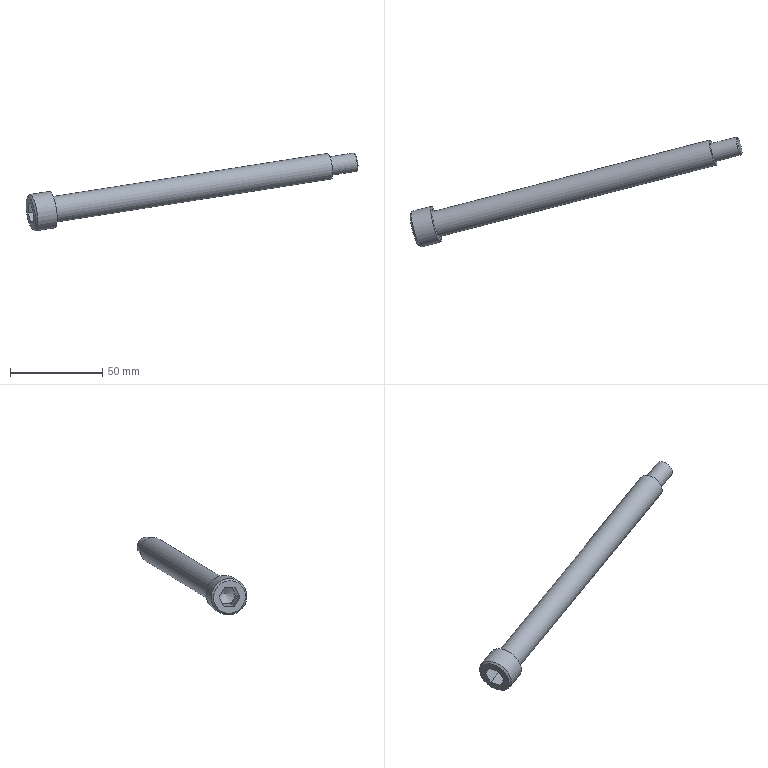Part | STEP file | 车灯-后视镜_id250_x_t | 1 solid | 23 faces | box 180.044 x 59.602 x 42.214 mm | volume 28311 mm3 | plane 17 | cylinder 3 | cone 3 | commonest cylinder face diameters 10 x1 14 x1 20 x1
STEP:
#1=CARTESIAN_POINT('',(-70.664,50.819,2.468));
#2=VERTEX_POINT('',#1);
#3=CARTESIAN_POINT('',(-69.54,46.461,2.468));
#4=DIRECTION('',(0.9573,0.2469,0.1502));
#5=DIRECTION('',(-0.2498,0.9683,0.));
#6=AXIS2_PLACEMENT_3D('',#3,#4,#5);
#7=CIRCLE('',#6,4.5);
#8=EDGE_CURVE('',#2,#2,#7,.T.);
#9=ORIENTED_EDGE('',*,*,#8,.T.);
#10=EDGE_LOOP('',(#9));
#11=FACE_OUTER_BOUND('',#10,.T.);
#12=CARTESIAN_POINT('',(-69.54,46.461,2.468));
#13=DIRECTION('',(0.9573,0.2469,0.1502));
#14=DIRECTION('',(-0.2498,0.9683,0.));
#15=AXIS2_PLACEMENT_3D('',#12,#13,#14);
#16=PLANE('',#15);
#17=ADVANCED_FACE('',(#11),#16,.T.);
#18=CARTESIAN_POINT('',(-85.149,47.599,0.216));
#19=VERTEX_POINT('',#18);
#20=CARTESIAN_POINT('',(-83.9,42.757,0.216));
#21=DIRECTION('',(-0.9573,-0.2469,-0.1502));
#22=DIRECTION('',(-0.2498,0.9683,0.));
#23=AXIS2_PLACEMENT_3D('',#20,#21,#22);
#24=CIRCLE('',#23,5.);
#25=EDGE_CURVE('',#19,#19,#24,.T.);
#26=ORIENTED_EDGE('',*,*,#25,.F.);
#27=EDGE_LOOP('',(#26));
#28=FACE_BOUND('',#27,.T.);
#29=CARTESIAN_POINT('',(-71.267,51.179,2.393));
#30=VERTEX_POINT('',#29);
#31=CARTESIAN_POINT('',(-70.019,46.338,2.393));
#32=DIRECTION('',(-0.9573,-0.2469,-0.1502));
#33=DIRECTION('',(-0.2498,0.9683,0.));
#34=AXIS2_PLACEMENT_3D('',#31,#32,#33);
#35=CIRCLE('',#34,5.);
#36=EDGE_CURVE('',#30,#30,#35,.T.);
#37=ORIENTED_EDGE('',*,*,#36,.T.);
#38=EDGE_LOOP('',(#37));
#39=FACE_BOUND('',#38,.T.);
#40=CARTESIAN_POINT('',(-88.686,41.523,-0.5348));
#41=DIRECTION('',(0.9573,0.2469,0.1502));
#42=DIRECTION('',(-0.2498,0.9683,0.));
#43=AXIS2_PLACEMENT_3D('',#40,#41,#42);
#44=CYLINDRICAL_SURFACE('',#43,5.);
#45=ADVANCED_FACE('',(#28,#39),#44,.T.);
#46=ORIENTED_EDGE('',*,*,#8,.F.);
#47=EDGE_LOOP('',(#46));
#48=FACE_BOUND('',#47,.T.);
#49=ORIENTED_EDGE('',*,*,#36,.F.);
#50=EDGE_LOOP('',(#49));
#51=FACE_BOUND('',#50,.T.);
#52=CARTESIAN_POINT('',(-70.019,46.338,2.393));
#53=DIRECTION('',(-0.9573,-0.2469,-0.1502));
#54=DIRECTION('',(0.2498,-0.9683,0.));
#55=AXIS2_PLACEMENT_3D('',#52,#53,#54);
#56=CONICAL_SURFACE('',#55,5.,45.);
#57=ADVANCED_FACE('',(#48,#51),#56,.T.);
#58=ORIENTED_EDGE('',*,*,#25,.T.);
#59=EDGE_LOOP('',(#58));
#60=FACE_BOUND('',#59,.T.);
#61=CARTESIAN_POINT('',(-85.648,49.535,0.216));
#62=VERTEX_POINT('',#61);
#63=CARTESIAN_POINT('',(-83.9,42.757,0.216));
#64=DIRECTION('',(-0.9573,-0.2469,-0.1502));
#65=DIRECTION('',(-0.2498,0.9683,0.));
#66=AXIS2_PLACEMENT_3D('',#63,#64,#65);
#67=CIRCLE('',#66,7.);
#68=EDGE_CURVE('',#62,#62,#67,.T.);
#69=ORIENTED_EDGE('',*,*,#68,.F.);
#70=EDGE_LOOP('',(#69));
#71=FACE_BOUND('',#70,.T.);
#72=CARTESIAN_POINT('',(-83.9,42.757,0.216));
#73=DIRECTION('',(0.9573,0.2469,0.1502));
#74=DIRECTION('',(-0.2498,0.9683,0.));
#75=AXIS2_PLACEMENT_3D('',#72,#73,#74);
#76=PLANE('',#75);
#77=ADVANCED_FACE('',(#60,#71),#76,.T.);
#78=CARTESIAN_POINT('',(-235.949,10.767,-23.358));
#79=VERTEX_POINT('',#78);
#80=CARTESIAN_POINT('',(-232.452,-2.79,-23.36));
#81=VERTEX_POINT('',#80);
#82=CARTESIAN_POINT('',(-234.2,3.988,-23.359));
#83=DIRECTION('',(0.9573,0.2469,0.1502));
#84=DIRECTION('',(-0.2498,0.9683,0.));
#85=AXIS2_PLACEMENT_3D('',#82,#83,#84);
#86=CIRCLE('',#85,7.);
#87=EDGE_CURVE('',#79,#81,#86,.T.);
#88=ORIENTED_EDGE('',*,*,#87,.T.);
#89=CARTESIAN_POINT('',(-234.2,3.988,-23.359));
#90=DIRECTION('',(0.9576,0.247,0.1481));
#91=DIRECTION('',(0.1433,0.03713,-0.989));
#92=AXIS2_PLACEMENT_3D('',#89,#90,#91);
#93=ELLIPSE('',#92,7.,7.);
#94=EDGE_CURVE('',#81,#79,#93,.T.);
#95=ORIENTED_EDGE('',*,*,#94,.T.);
#96=EDGE_LOOP('',(#88,#95));
#97=FACE_BOUND('',#96,.T.);
#98=ORIENTED_EDGE('',*,*,#68,.T.);
#99=EDGE_LOOP('',(#98));
#100=FACE_BOUND('',#99,.T.);
#101=CARTESIAN_POINT('',(-88.686,41.523,-0.5348));
#102=DIRECTION('',(-0.9573,-0.2469,-0.1502));
#103=DIRECTION('',(0.2498,-0.9683,0.));
#104=AXIS2_PLACEMENT_3D('',#101,#102,#103);
#105=CYLINDRICAL_SURFACE('',#104,7.);
#106=ADVANCED_FACE('',(#97,#100),#105,.T.);
#107=CARTESIAN_POINT('',(-236.698,13.671,-23.358));
#108=VERTEX_POINT('',#107);
#109=CARTESIAN_POINT('',(-231.702,-5.695,-23.361));
#110=VERTEX_POINT('',#109);
#111=CARTESIAN_POINT('',(-234.2,3.988,-23.359));
#112=DIRECTION('',(-0.9576,-0.247,-0.1481));
#113=DIRECTION('',(-0.2498,0.9683,-0.00001827));
#114=AXIS2_PLACEMENT_3D('',#111,#112,#113);
#115=CIRCLE('',#114,10.);
#116=EDGE_CURVE('',#108,#110,#115,.T.);
#117=ORIENTED_EDGE('',*,*,#116,.F.);
#118=CARTESIAN_POINT('',(-234.2,3.988,-23.359));
#119=DIRECTION('',(0.2498,-0.9683,-0.0001518));
#120=VECTOR('',#119,1.);
#121=LINE('',#118,#120);
#122=EDGE_CURVE('',#108,#79,#121,.T.);
#123=ORIENTED_EDGE('',*,*,#122,.T.);
#124=ORIENTED_EDGE('',*,*,#94,.F.);
#125=CARTESIAN_POINT('',(-234.2,3.988,-23.359));
#126=DIRECTION('',(0.2498,-0.9683,-0.0001518));
#127=VECTOR('',#126,1.);
#128=LINE('',#125,#127);
#129=EDGE_CURVE('',#81,#110,#128,.T.);
#130=ORIENTED_EDGE('',*,*,#129,.T.);
#131=EDGE_LOOP('',(#117,#123,#124,#130));
#132=FACE_OUTER_BOUND('',#131,.T.);
#133=CARTESIAN_POINT('',(-234.2,3.988,-23.359));
#134=DIRECTION('',(0.9576,0.247,0.1481));
#135=DIRECTION('',(-0.2498,0.9683,-0.00001827));
#136=AXIS2_PLACEMENT_3D('',#133,#134,#135);
#137=PLANE('',#136);
#138=ADVANCED_FACE('',(#132),#137,.T.);
#139=CARTESIAN_POINT('',(-242.236,-8.412,-24.988));
#140=VERTEX_POINT('',#139);
#141=CARTESIAN_POINT('',(-244.734,1.271,-24.988));
#142=DIRECTION('',(0.9576,0.247,0.1481));
#143=DIRECTION('',(0.2498,-0.9683,0.00001827));
#144=AXIS2_PLACEMENT_3D('',#141,#142,#143);
#145=CIRCLE('',#144,10.);
#146=EDGE_CURVE('',#140,#140,#145,.T.);
#147=ORIENTED_EDGE('',*,*,#146,.T.);
#148=EDGE_LOOP('',(#147));
#149=FACE_BOUND('',#148,.T.);
#150=ORIENTED_EDGE('',*,*,#116,.T.);
#151=CARTESIAN_POINT('',(-234.2,3.988,-23.359));
#152=DIRECTION('',(-0.9573,-0.2469,-0.1502));
#153=DIRECTION('',(-0.1454,-0.03765,0.9887));
#154=AXIS2_PLACEMENT_3D('',#151,#152,#153);
#155=ELLIPSE('',#154,10.,10.);
#156=EDGE_CURVE('',#110,#108,#155,.T.);
#157=ORIENTED_EDGE('',*,*,#156,.T.);
#158=EDGE_LOOP('',(#150,#157));
#159=FACE_BOUND('',#158,.T.);
#160=CARTESIAN_POINT('',(-238.988,2.753,-24.099));
#161=DIRECTION('',(-0.9576,-0.247,-0.1481));
#162=DIRECTION('',(0.2498,-0.9683,0.00001827));
#163=AXIS2_PLACEMENT_3D('',#160,#161,#162);
#164=CYLINDRICAL_SURFACE('',#163,10.);
#165=ADVANCED_FACE('',(#149,#159),#164,.T.);
#166=CARTESIAN_POINT('',(-237.308,-1.285,-21.479));
#167=VERTEX_POINT('',#166);
#168=CARTESIAN_POINT('',(-238.747,2.816,-19.006));
#169=VERTEX_POINT('',#168);
#170=CARTESIAN_POINT('',(-238.031,3.,-23.951));
#171=DIRECTION('',(-0.9576,-0.247,-0.1481));
#172=DIRECTION('',(0.2498,-0.9683,0.00001827));
#173=AXIS2_PLACEMENT_3D('',#170,#171,#172);
#174=CIRCLE('',#173,5.);
#175=EDGE_CURVE('',#167,#169,#174,.T.);
#176=ORIENTED_EDGE('',*,*,#175,.F.);
#177=CARTESIAN_POINT('',(-238.026,0.02036,-19.006));
#178=VERTEX_POINT('',#177);
#179=CARTESIAN_POINT('',(-236.589,-2.59,-23.951));
#180=DIRECTION('',(-0.249,0.4521,0.8565));
#181=VECTOR('',#180,1.);
#182=LINE('',#179,#181);
#183=EDGE_CURVE('',#167,#178,#182,.T.);
#184=ORIENTED_EDGE('',*,*,#183,.T.);
#185=CARTESIAN_POINT('',(-238.026,0.02036,-19.006));
#186=DIRECTION('',(-0.2498,0.9683,-0.00001827));
#187=VECTOR('',#186,1.);
#188=LINE('',#185,#187);
#189=EDGE_CURVE('',#178,#169,#188,.T.);
#190=ORIENTED_EDGE('',*,*,#189,.T.);
#191=EDGE_LOOP('',(#176,#184,#190));
#192=FACE_OUTER_BOUND('',#191,.T.);
#193=CARTESIAN_POINT('',(-240.911,11.201,-19.007));
#194=DIRECTION('',(-0.9576,-0.247,-0.1481));
#195=DIRECTION('',(0.2498,-0.9683,0.00001827));
#196=AXIS2_PLACEMENT_3D('',#193,#194,#195);
#197=PLANE('',#196);
#198=ADVANCED_FACE('',(#192),#197,.T.);
#199=CARTESIAN_POINT('',(-239.471,7.101,-21.479));
#200=VERTEX_POINT('',#199);
#201=CARTESIAN_POINT('',(-238.031,3.,-23.951));
#202=DIRECTION('',(-0.9576,-0.247,-0.1481));
#203=DIRECTION('',(0.2498,-0.9683,0.00001827));
#204=AXIS2_PLACEMENT_3D('',#201,#202,#203);
#205=CIRCLE('',#204,5.);
#206=EDGE_CURVE('',#169,#200,#205,.T.);
#207=ORIENTED_EDGE('',*,*,#206,.F.);
#208=CARTESIAN_POINT('',(-239.468,5.611,-19.007));
#209=VERTEX_POINT('',#208);
#210=CARTESIAN_POINT('',(-238.026,0.02036,-19.006));
#211=DIRECTION('',(-0.2498,0.9683,-0.00001827));
#212=VECTOR('',#211,1.);
#213=LINE('',#210,#212);
#214=EDGE_CURVE('',#169,#209,#213,.T.);
#215=ORIENTED_EDGE('',*,*,#214,.T.);
#216=CARTESIAN_POINT('',(-239.468,5.611,-19.007));
#217=DIRECTION('',(-0.0007198,0.5162,-0.8565));
#218=VECTOR('',#217,1.);
#219=LINE('',#216,#218);
#220=EDGE_CURVE('',#209,#200,#219,.T.);
#221=ORIENTED_EDGE('',*,*,#220,.T.);
#222=EDGE_LOOP('',(#207,#215,#221));
#223=FACE_OUTER_BOUND('',#222,.T.);
#224=CARTESIAN_POINT('',(-240.911,11.201,-19.007));
#225=DIRECTION('',(-0.9576,-0.247,-0.1481));
#226=DIRECTION('',(0.2498,-0.9683,0.00001827));
#227=AXIS2_PLACEMENT_3D('',#224,#225,#226);
#228=PLANE('',#227);
#229=ADVANCED_FACE('',(#223),#228,.T.);
#230=CARTESIAN_POINT('',(-238.754,7.286,-26.424));
#231=VERTEX_POINT('',#230);
#232=CARTESIAN_POINT('',(-238.031,3.,-23.951));
#233=DIRECTION('',(-0.9576,-0.247,-0.1481));
#234=DIRECTION('',(0.2498,-0.9683,0.00001827));
#235=AXIS2_PLACEMENT_3D('',#232,#233,#234);
#236=CIRCLE('',#235,5.);
#237=EDGE_CURVE('',#200,#231,#236,.T.);
#238=ORIENTED_EDGE('',*,*,#237,.F.);
#239=CARTESIAN_POINT('',(-239.473,8.591,-23.951));
#240=VERTEX_POINT('',#239);
#241=CARTESIAN_POINT('',(-239.468,5.611,-19.007));
#242=DIRECTION('',(-0.0007198,0.5162,-0.8565));
#243=VECTOR('',#242,1.);
#244=LINE('',#241,#243);
#245=EDGE_CURVE('',#200,#240,#244,.T.);
#246=ORIENTED_EDGE('',*,*,#245,.T.);
#247=CARTESIAN_POINT('',(-239.473,8.591,-23.951));
#248=DIRECTION('',(0.249,-0.4521,-0.8565));
#249=VECTOR('',#248,1.);
#250=LINE('',#247,#249);
#251=EDGE_CURVE('',#240,#231,#250,.T.);
#252=ORIENTED_EDGE('',*,*,#251,.T.);
#253=EDGE_LOOP('',(#238,#246,#252));
#254=FACE_OUTER_BOUND('',#253,.T.);
#255=CARTESIAN_POINT('',(-240.911,11.201,-19.007));
#256=DIRECTION('',(-0.9576,-0.247,-0.1481));
#257=DIRECTION('',(0.2498,-0.9683,0.00001827));
#258=AXIS2_PLACEMENT_3D('',#255,#256,#257);
#259=PLANE('',#258);
#260=ADVANCED_FACE('',(#254),#259,.T.);
#261=CARTESIAN_POINT('',(-237.314,3.185,-28.896));
#262=VERTEX_POINT('',#261);
#263=CARTESIAN_POINT('',(-238.031,3.,-23.951));
#264=DIRECTION('',(-0.9576,-0.247,-0.1481));
#265=DIRECTION('',(-0.2498,0.9683,-0.00001827));
#266=AXIS2_PLACEMENT_3D('',#263,#264,#265);
#267=CIRCLE('',#266,5.);
#268=EDGE_CURVE('',#231,#262,#267,.T.);
#269=ORIENTED_EDGE('',*,*,#268,.F.);
#270=CARTESIAN_POINT('',(-238.035,5.981,-28.896));
#271=VERTEX_POINT('',#270);
#272=CARTESIAN_POINT('',(-239.473,8.591,-23.951));
#273=DIRECTION('',(0.249,-0.4521,-0.8565));
#274=VECTOR('',#273,1.);
#275=LINE('',#272,#274);
#276=EDGE_CURVE('',#231,#271,#275,.T.);
#277=ORIENTED_EDGE('',*,*,#276,.T.);
#278=CARTESIAN_POINT('',(-238.035,5.981,-28.896));
#279=DIRECTION('',(0.2498,-0.9683,0.00001827));
#280=VECTOR('',#279,1.);
#281=LINE('',#278,#280);
#282=EDGE_CURVE('',#271,#262,#281,.T.);
#283=ORIENTED_EDGE('',*,*,#282,.T.);
#284=EDGE_LOOP('',(#269,#277,#283));
#285=FACE_OUTER_BOUND('',#284,.T.);
#286=CARTESIAN_POINT('',(-240.911,11.201,-19.007));
#287=DIRECTION('',(-0.9576,-0.247,-0.1481));
#288=DIRECTION('',(0.2498,-0.9683,0.00001827));
#289=AXIS2_PLACEMENT_3D('',#286,#287,#288);
#290=PLANE('',#289);
#291=ADVANCED_FACE('',(#285),#290,.T.);
#292=CARTESIAN_POINT('',(-236.591,-1.1,-26.424));
#293=VERTEX_POINT('',#292);
#294=CARTESIAN_POINT('',(-238.031,3.,-23.951));
#295=DIRECTION('',(-0.9576,-0.247,-0.1481));
#296=DIRECTION('',(0.2498,-0.9683,0.00001827));
#297=AXIS2_PLACEMENT_3D('',#294,#295,#296);
#298=CIRCLE('',#297,5.);
#299=EDGE_CURVE('',#262,#293,#298,.T.);
#300=ORIENTED_EDGE('',*,*,#299,.F.);
#301=CARTESIAN_POINT('',(-236.593,0.39,-28.896));
#302=VERTEX_POINT('',#301);
#303=CARTESIAN_POINT('',(-238.035,5.981,-28.896));
#304=DIRECTION('',(0.2498,-0.9683,0.00001827));
#305=VECTOR('',#304,1.);
#306=LINE('',#303,#305);
#307=EDGE_CURVE('',#262,#302,#306,.T.);
#308=ORIENTED_EDGE('',*,*,#307,.T.);
#309=CARTESIAN_POINT('',(-236.593,0.39,-28.896));
#310=DIRECTION('',(0.0007198,-0.5162,0.8565));
#311=VECTOR('',#310,1.);
#312=LINE('',#309,#311);
#313=EDGE_CURVE('',#302,#293,#312,.T.);
#314=ORIENTED_EDGE('',*,*,#313,.T.);
#315=EDGE_LOOP('',(#300,#308,#314));
#316=FACE_OUTER_BOUND('',#315,.T.);
#317=CARTESIAN_POINT('',(-240.911,11.201,-19.007));
#318=DIRECTION('',(-0.9576,-0.247,-0.1481));
#319=DIRECTION('',(0.2498,-0.9683,0.00001827));
#320=AXIS2_PLACEMENT_3D('',#317,#318,#319);
#321=PLANE('',#320);
#322=ADVANCED_FACE('',(#316),#321,.T.);
#323=CARTESIAN_POINT('',(-243.444,-7.69,-25.136));
#324=VERTEX_POINT('',#323);
#325=CARTESIAN_POINT('',(-245.692,1.024,-25.136));
#326=DIRECTION('',(-0.9576,-0.247,-0.1481));
#327=DIRECTION('',(0.2498,-0.9683,0.00001827));
#328=AXIS2_PLACEMENT_3D('',#325,#326,#327);
#329=CIRCLE('',#328,9.);
#330=EDGE_CURVE('',#324,#324,#329,.T.);
#331=ORIENTED_EDGE('',*,*,#330,.T.);
#332=EDGE_LOOP('',(#331));
#333=FACE_BOUND('',#332,.T.);
#334=CARTESIAN_POINT('',(-245.688,-1.956,-20.191));
#335=VERTEX_POINT('',#334);
#336=CARTESIAN_POINT('',(-247.13,3.635,-20.191));
#337=VERTEX_POINT('',#336);
#338=CARTESIAN_POINT('',(-245.688,-1.956,-20.191));
#339=DIRECTION('',(-0.2498,0.9683,-0.00001827));
#340=VECTOR('',#339,1.);
#341=LINE('',#338,#340);
#342=EDGE_CURVE('',#335,#337,#341,.T.);
#343=ORIENTED_EDGE('',*,*,#342,.F.);
#344=CARTESIAN_POINT('',(-244.25,-4.566,-25.136));
#345=VERTEX_POINT('',#344);
#346=CARTESIAN_POINT('',(-244.25,-4.566,-25.136));
#347=DIRECTION('',(-0.249,0.4521,0.8565));
#348=VECTOR('',#347,1.);
#349=LINE('',#346,#348);
#350=EDGE_CURVE('',#345,#335,#349,.T.);
#351=ORIENTED_EDGE('',*,*,#350,.F.);
#352=CARTESIAN_POINT('',(-244.254,-1.586,-30.081));
#353=VERTEX_POINT('',#352);
#354=CARTESIAN_POINT('',(-244.254,-1.586,-30.081));
#355=DIRECTION('',(0.0007198,-0.5162,0.8565));
#356=VECTOR('',#355,1.);
#357=LINE('',#354,#356);
#358=EDGE_CURVE('',#353,#345,#357,.T.);
#359=ORIENTED_EDGE('',*,*,#358,.F.);
#360=CARTESIAN_POINT('',(-245.696,4.004,-30.081));
#361=VERTEX_POINT('',#360);
#362=CARTESIAN_POINT('',(-245.696,4.004,-30.081));
#363=DIRECTION('',(0.2498,-0.9683,0.00001827));
#364=VECTOR('',#363,1.);
#365=LINE('',#362,#364);
#366=EDGE_CURVE('',#361,#353,#365,.T.);
#367=ORIENTED_EDGE('',*,*,#366,.F.);
#368=CARTESIAN_POINT('',(-247.134,6.615,-25.136));
#369=VERTEX_POINT('',#368);
#370=CARTESIAN_POINT('',(-247.134,6.615,-25.136));
#371=DIRECTION('',(0.249,-0.4521,-0.8565));
#372=VECTOR('',#371,1.);
#373=LINE('',#370,#372);
#374=EDGE_CURVE('',#369,#361,#373,.T.);
#375=ORIENTED_EDGE('',*,*,#374,.F.);
#376=CARTESIAN_POINT('',(-247.13,3.635,-20.191));
#377=DIRECTION('',(-0.0007198,0.5162,-0.8565));
#378=VECTOR('',#377,1.);
#379=LINE('',#376,#378);
#380=EDGE_CURVE('',#337,#369,#379,.T.);
#381=ORIENTED_EDGE('',*,*,#380,.F.);
#382=EDGE_LOOP('',(#343,#351,#359,#367,#375,#381));
#383=FACE_BOUND('',#382,.T.);
#384=CARTESIAN_POINT('',(-245.692,1.024,-25.136));
#385=DIRECTION('',(-0.9576,-0.247,-0.1481));
#386=DIRECTION('',(0.2498,-0.9683,0.00001827));
#387=AXIS2_PLACEMENT_3D('',#384,#385,#386);
#388=PLANE('',#387);
#389=ADVANCED_FACE('',(#333,#383),#388,.T.);
#390=ORIENTED_EDGE('',*,*,#342,.T.);
#391=CARTESIAN_POINT('',(-239.468,5.611,-19.007));
#392=DIRECTION('',(-0.9576,-0.247,-0.1481));
#393=VECTOR('',#392,1.);
#394=LINE('',#391,#393);
#395=EDGE_CURVE('',#209,#337,#394,.T.);
#396=ORIENTED_EDGE('',*,*,#395,.F.);
#397=ORIENTED_EDGE('',*,*,#214,.F.);
#398=ORIENTED_EDGE('',*,*,#189,.F.);
#399=CARTESIAN_POINT('',(-238.026,0.02036,-19.006));
#400=DIRECTION('',(-0.9576,-0.247,-0.1481));
#401=VECTOR('',#400,1.);
#402=LINE('',#399,#401);
#403=EDGE_CURVE('',#178,#335,#402,.T.);
#404=ORIENTED_EDGE('',*,*,#403,.T.);
#405=EDGE_LOOP('',(#390,#396,#397,#398,#404));
#406=FACE_OUTER_BOUND('',#405,.T.);
#407=CARTESIAN_POINT('',(-238.026,0.02036,-19.006));
#408=DIRECTION('',(-0.1434,-0.03696,0.989));
#409=DIRECTION('',(0.9897,-0.001118,0.1434));
#410=AXIS2_PLACEMENT_3D('',#407,#408,#409);
#411=PLANE('',#410);
#412=ADVANCED_FACE('',(#406),#411,.F.);
#413=ORIENTED_EDGE('',*,*,#380,.T.);
#414=CARTESIAN_POINT('',(-239.473,8.591,-23.951));
#415=DIRECTION('',(-0.9576,-0.247,-0.1481));
#416=VECTOR('',#415,1.);
#417=LINE('',#414,#416);
#418=EDGE_CURVE('',#240,#369,#417,.T.);
#419=ORIENTED_EDGE('',*,*,#418,.F.);
#420=ORIENTED_EDGE('',*,*,#245,.F.);
#421=ORIENTED_EDGE('',*,*,#220,.F.);
#422=ORIENTED_EDGE('',*,*,#395,.T.);
#423=EDGE_LOOP('',(#413,#419,#420,#421,#422));
#424=FACE_OUTER_BOUND('',#423,.T.);
#425=CARTESIAN_POINT('',(-239.468,5.611,-19.007));
#426=DIRECTION('',(-0.288,0.8201,0.4945));
#427=DIRECTION('',(-0.2124,-0.5582,0.8021));
#428=AXIS2_PLACEMENT_3D('',#425,#426,#427);
#429=PLANE('',#428);
#430=ADVANCED_FACE('',(#424),#429,.F.);
#431=ORIENTED_EDGE('',*,*,#374,.T.);
#432=CARTESIAN_POINT('',(-238.035,5.981,-28.896));
#433=DIRECTION('',(-0.9576,-0.247,-0.1481));
#434=VECTOR('',#433,1.);
#435=LINE('',#432,#434);
#436=EDGE_CURVE('',#271,#361,#435,.T.);
#437=ORIENTED_EDGE('',*,*,#436,.F.);
#438=ORIENTED_EDGE('',*,*,#276,.F.);
#439=ORIENTED_EDGE('',*,*,#251,.F.);
#440=ORIENTED_EDGE('',*,*,#418,.T.);
#441=EDGE_LOOP('',(#431,#437,#438,#439,#440));
#442=FACE_OUTER_BOUND('',#441,.T.);
#443=CARTESIAN_POINT('',(-239.473,8.591,-23.951));
#444=DIRECTION('',(-0.1446,0.8571,-0.4945));
#445=DIRECTION('',(-0.2189,0.4597,0.8607));
#446=AXIS2_PLACEMENT_3D('',#443,#444,#445);
#447=PLANE('',#446);
#448=ADVANCED_FACE('',(#442),#447,.F.);
#449=ORIENTED_EDGE('',*,*,#366,.T.);
#450=CARTESIAN_POINT('',(-236.593,0.39,-28.896));
#451=DIRECTION('',(-0.9576,-0.247,-0.1481));
#452=VECTOR('',#451,1.);
#453=LINE('',#450,#452);
#454=EDGE_CURVE('',#302,#353,#453,.T.);
#455=ORIENTED_EDGE('',*,*,#454,.F.);
#456=ORIENTED_EDGE('',*,*,#307,.F.);
#457=ORIENTED_EDGE('',*,*,#282,.F.);
#458=ORIENTED_EDGE('',*,*,#436,.T.);
#459=EDGE_LOOP('',(#449,#455,#456,#457,#458));
#460=FACE_OUTER_BOUND('',#459,.T.);
#461=CARTESIAN_POINT('',(-238.035,5.981,-28.896));
#462=DIRECTION('',(0.1434,0.03696,-0.989));
#463=DIRECTION('',(-0.9897,0.001118,-0.1434));
#464=AXIS2_PLACEMENT_3D('',#461,#462,#463);
#465=PLANE('',#464);
#466=ADVANCED_FACE('',(#460),#465,.F.);
#467=ORIENTED_EDGE('',*,*,#358,.T.);
#468=CARTESIAN_POINT('',(-236.589,-2.59,-23.951));
#469=VERTEX_POINT('',#468);
#470=CARTESIAN_POINT('',(-236.589,-2.59,-23.951));
#471=DIRECTION('',(-0.9576,-0.247,-0.1481));
#472=VECTOR('',#471,1.);
#473=LINE('',#470,#472);
#474=EDGE_CURVE('',#469,#345,#473,.T.);
#475=ORIENTED_EDGE('',*,*,#474,.F.);
#476=CARTESIAN_POINT('',(-236.593,0.39,-28.896));
#477=DIRECTION('',(0.0007198,-0.5162,0.8565));
#478=VECTOR('',#477,1.);
#479=LINE('',#476,#478);
#480=EDGE_CURVE('',#293,#469,#479,.T.);
#481=ORIENTED_EDGE('',*,*,#480,.F.);
#482=ORIENTED_EDGE('',*,*,#313,.F.);
#483=ORIENTED_EDGE('',*,*,#454,.T.);
#484=EDGE_LOOP('',(#467,#475,#481,#482,#483));
#485=FACE_OUTER_BOUND('',#484,.T.);
#486=CARTESIAN_POINT('',(-236.593,0.39,-28.896));
#487=DIRECTION('',(0.288,-0.8201,-0.4945));
#488=DIRECTION('',(0.2124,0.5582,-0.8021));
#489=AXIS2_PLACEMENT_3D('',#486,#487,#488);
#490=PLANE('',#489);
#491=ADVANCED_FACE('',(#485),#490,.F.);
#492=ORIENTED_EDGE('',*,*,#350,.T.);
#493=ORIENTED_EDGE('',*,*,#403,.F.);
#494=ORIENTED_EDGE('',*,*,#183,.F.);
#495=CARTESIAN_POINT('',(-236.589,-2.59,-23.951));
#496=DIRECTION('',(-0.249,0.4521,0.8565));
#497=VECTOR('',#496,1.);
#498=LINE('',#495,#497);
#499=EDGE_CURVE('',#469,#167,#498,.T.);
#500=ORIENTED_EDGE('',*,*,#499,.F.);
#501=ORIENTED_EDGE('',*,*,#474,.T.);
#502=EDGE_LOOP('',(#492,#493,#494,#500,#501));
#503=FACE_OUTER_BOUND('',#502,.T.);
#504=CARTESIAN_POINT('',(-236.589,-2.59,-23.951));
#505=DIRECTION('',(0.1446,-0.8571,0.4945));
#506=DIRECTION('',(0.2189,-0.4597,-0.8607));
#507=AXIS2_PLACEMENT_3D('',#504,#505,#506);
#508=PLANE('',#507);
#509=ADVANCED_FACE('',(#503),#508,.F.);
#510=CARTESIAN_POINT('',(-238.031,3.,-23.951));
#511=DIRECTION('',(-0.9576,-0.247,-0.1481));
#512=DIRECTION('',(0.2498,-0.9683,0.00001827));
#513=AXIS2_PLACEMENT_3D('',#510,#511,#512);
#514=CIRCLE('',#513,5.);
#515=EDGE_CURVE('',#293,#167,#514,.T.);
#516=ORIENTED_EDGE('',*,*,#515,.F.);
#517=ORIENTED_EDGE('',*,*,#480,.T.);
#518=ORIENTED_EDGE('',*,*,#499,.T.);
#519=EDGE_LOOP('',(#516,#517,#518));
#520=FACE_OUTER_BOUND('',#519,.T.);
#521=CARTESIAN_POINT('',(-240.911,11.201,-19.007));
#522=DIRECTION('',(-0.9576,-0.247,-0.1481));
#523=DIRECTION('',(0.2498,-0.9683,0.00001827));
#524=AXIS2_PLACEMENT_3D('',#521,#522,#523);
#525=PLANE('',#524);
#526=ADVANCED_FACE('',(#520),#525,.T.);
#527=CARTESIAN_POINT('',(-235.158,3.741,-23.507));
#528=VERTEX_POINT('',#527);
#529=VERTEX_LOOP('',#528);
#530=FACE_BOUND('',#529,.T.);
#531=ORIENTED_EDGE('',*,*,#268,.T.);
#532=ORIENTED_EDGE('',*,*,#299,.T.);
#533=ORIENTED_EDGE('',*,*,#515,.T.);
#534=ORIENTED_EDGE('',*,*,#175,.T.);
#535=ORIENTED_EDGE('',*,*,#206,.T.);
#536=ORIENTED_EDGE('',*,*,#237,.T.);
#537=EDGE_LOOP('',(#531,#532,#533,#534,#535,#536));
#538=FACE_BOUND('',#537,.T.);
#539=CARTESIAN_POINT('',(-238.031,3.,-23.951));
#540=DIRECTION('',(-0.9576,-0.247,-0.1481));
#541=DIRECTION('',(0.2498,-0.9683,0.00001827));
#542=AXIS2_PLACEMENT_3D('',#539,#540,#541);
#543=CONICAL_SURFACE('',#542,5.,59.036);
#544=ADVANCED_FACE('',(#530,#538),#543,.F.);
#545=ORIENTED_EDGE('',*,*,#330,.F.);
#546=EDGE_LOOP('',(#545));
#547=FACE_BOUND('',#546,.T.);
#548=ORIENTED_EDGE('',*,*,#146,.F.);
#549=EDGE_LOOP('',(#548));
#550=FACE_BOUND('',#549,.T.);
#551=CARTESIAN_POINT('',(-244.734,1.271,-24.988));
#552=DIRECTION('',(0.9576,0.247,0.1481));
#553=DIRECTION('',(-0.2498,0.9683,-0.00001827));
#554=AXIS2_PLACEMENT_3D('',#551,#552,#553);
#555=CONICAL_SURFACE('',#554,10.,45.);
#556=ADVANCED_FACE('',(#547,#550),#555,.T.);
#557=ORIENTED_EDGE('',*,*,#129,.F.);
#558=ORIENTED_EDGE('',*,*,#87,.F.);
#559=ORIENTED_EDGE('',*,*,#122,.F.);
#560=ORIENTED_EDGE('',*,*,#156,.F.);
#561=EDGE_LOOP('',(#557,#558,#559,#560));
#562=FACE_OUTER_BOUND('',#561,.T.);
#563=CARTESIAN_POINT('',(-234.2,3.988,-23.359));
#564=DIRECTION('',(0.9573,0.2469,0.1502));
#565=DIRECTION('',(-0.2498,0.9683,0.));
#566=AXIS2_PLACEMENT_3D('',#563,#564,#565);
#567=PLANE('',#566);
#568=ADVANCED_FACE('',(#562),#567,.T.);
#569=CLOSED_SHELL('',(#17,#45,#57,#77,#106,#138,#165,#198,#229,#260,#291,#322,#389,#412,#430,#448,#466,#491,#509,#526,#544,#556,#568));
#570=MANIFOLD_SOLID_BREP('',#569);
#571=(LENGTH_UNIT()NAMED_UNIT(*)SI_UNIT(.MILLI.,.METRE.));
#572=UNCERTAINTY_MEASURE_WITH_UNIT(LENGTH_MEASURE(0.03555),#571,'','');
#573=(NAMED_UNIT(*)PLANE_ANGLE_UNIT()SI_UNIT($,.RADIAN.));
#574=PLANE_ANGLE_MEASURE_WITH_UNIT(PLANE_ANGLE_MEASURE(0.01745),#573);
#575=DIMENSIONAL_EXPONENTS(0.,0.,0.,0.,0.,0.,0.);
#576=(CONVERSION_BASED_UNIT('DEGREE',#574)NAMED_UNIT(#575)PLANE_ANGLE_UNIT());
#577=(NAMED_UNIT(*)SI_UNIT($,.STERADIAN.)SOLID_ANGLE_UNIT());
#578=(GEOMETRIC_REPRESENTATION_CONTEXT(3)GLOBAL_UNCERTAINTY_ASSIGNED_CONTEXT((#572))GLOBAL_UNIT_ASSIGNED_CONTEXT((#571,#576,#577))REPRESENTATION_CONTEXT('',''));
#579=ADVANCED_BREP_SHAPE_REPRESENTATION('',(#570),#578);